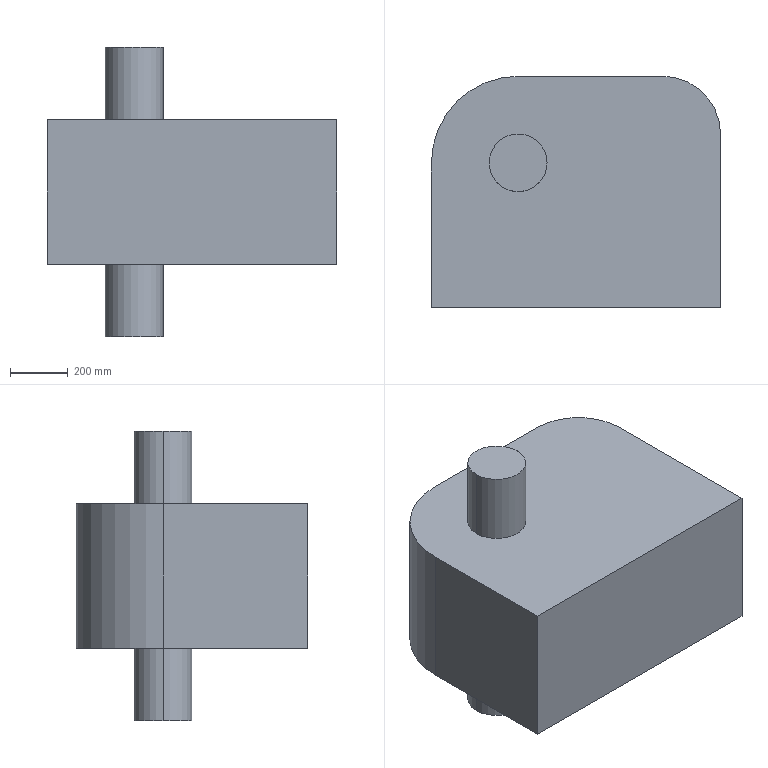Part | SolidWorks | features Fillet 2, Extrusion 1, ICE 1 | 1 solid | 14 faces | box 1000 x 800 x 1000 mm | volume 401758844 mm3 | plane 8 | cylinder 6 | commonest cylinder face diameters 200 x4 400 x1 600 x1
STEP:
#1=CARTESIAN_POINT('',(100.,0.,250.));
#2=VERTEX_POINT('',#1);
#3=CARTESIAN_POINT('',(-100.,0.,250.));
#4=VERTEX_POINT('',#3);
#5=CARTESIAN_POINT('',(0.,0.,250.));
#6=DIRECTION('',(0.,0.,1.));
#7=DIRECTION('',(1.,0.,0.));
#8=AXIS2_PLACEMENT_3D('',#5,#6,#7);
#9=CIRCLE('',#8,100.);
#10=EDGE_CURVE('',#2,#4,#9,.T.);
#11=ORIENTED_EDGE('',*,*,#10,.T.);
#12=CARTESIAN_POINT('',(-100.,0.,500.));
#13=VERTEX_POINT('',#12);
#14=CARTESIAN_POINT('',(-100.,0.,-500.));
#15=DIRECTION('',(0.,0.,1.));
#16=VECTOR('',#15,1000.);
#17=LINE('',#14,#16);
#18=EDGE_CURVE('',#4,#13,#17,.T.);
#19=ORIENTED_EDGE('',*,*,#18,.T.);
#20=CARTESIAN_POINT('',(100.,0.,500.));
#21=VERTEX_POINT('',#20);
#22=CARTESIAN_POINT('',(0.,0.,500.));
#23=DIRECTION('',(0.,0.,1.));
#24=DIRECTION('',(1.,0.,0.));
#25=AXIS2_PLACEMENT_3D('',#22,#23,#24);
#26=CIRCLE('',#25,100.);
#27=EDGE_CURVE('',#21,#13,#26,.T.);
#28=ORIENTED_EDGE('',*,*,#27,.F.);
#29=CARTESIAN_POINT('',(100.,0.,-500.));
#30=DIRECTION('',(0.,0.,1.));
#31=VECTOR('',#30,1000.);
#32=LINE('',#29,#31);
#33=EDGE_CURVE('',#2,#21,#32,.T.);
#34=ORIENTED_EDGE('',*,*,#33,.F.);
#35=EDGE_LOOP('',(#11,#19,#28,#34));
#36=FACE_OUTER_BOUND('',#35,.T.);
#37=CARTESIAN_POINT('',(0.,0.,-500.));
#38=DIRECTION('',(0.,0.,1.));
#39=DIRECTION('',(1.,0.,0.));
#40=AXIS2_PLACEMENT_3D('',#37,#38,#39);
#41=CYLINDRICAL_SURFACE('',#40,100.);
#42=ADVANCED_FACE('',(#36),#41,.T.);
#43=CARTESIAN_POINT('',(100.,0.,-500.));
#44=VERTEX_POINT('',#43);
#45=CARTESIAN_POINT('',(-100.,0.,-500.));
#46=VERTEX_POINT('',#45);
#47=CARTESIAN_POINT('',(0.,0.,-500.));
#48=DIRECTION('',(0.,0.,1.));
#49=DIRECTION('',(1.,0.,0.));
#50=AXIS2_PLACEMENT_3D('',#47,#48,#49);
#51=CIRCLE('',#50,100.);
#52=EDGE_CURVE('',#44,#46,#51,.T.);
#53=ORIENTED_EDGE('',*,*,#52,.T.);
#54=CARTESIAN_POINT('',(-100.,0.,-250.));
#55=VERTEX_POINT('',#54);
#56=CARTESIAN_POINT('',(-100.,0.,-500.));
#57=DIRECTION('',(0.,0.,1.));
#58=VECTOR('',#57,1000.);
#59=LINE('',#56,#58);
#60=EDGE_CURVE('',#46,#55,#59,.T.);
#61=ORIENTED_EDGE('',*,*,#60,.T.);
#62=CARTESIAN_POINT('',(100.,0.,-250.));
#63=VERTEX_POINT('',#62);
#64=CARTESIAN_POINT('',(0.,0.,-250.));
#65=DIRECTION('',(0.,0.,1.));
#66=DIRECTION('',(1.,0.,0.));
#67=AXIS2_PLACEMENT_3D('',#64,#65,#66);
#68=CIRCLE('',#67,100.);
#69=EDGE_CURVE('',#63,#55,#68,.T.);
#70=ORIENTED_EDGE('',*,*,#69,.F.);
#71=CARTESIAN_POINT('',(100.,0.,-500.));
#72=DIRECTION('',(0.,0.,1.));
#73=VECTOR('',#72,1000.);
#74=LINE('',#71,#73);
#75=EDGE_CURVE('',#44,#63,#74,.T.);
#76=ORIENTED_EDGE('',*,*,#75,.F.);
#77=EDGE_LOOP('',(#53,#61,#70,#76));
#78=FACE_OUTER_BOUND('',#77,.T.);
#79=CARTESIAN_POINT('',(0.,0.,-500.));
#80=DIRECTION('',(0.,0.,1.));
#81=DIRECTION('',(1.,0.,0.));
#82=AXIS2_PLACEMENT_3D('',#79,#80,#81);
#83=CYLINDRICAL_SURFACE('',#82,100.);
#84=ADVANCED_FACE('',(#78),#83,.T.);
#85=CARTESIAN_POINT('',(-300.,0.,250.));
#86=VERTEX_POINT('',#85);
#87=CARTESIAN_POINT('',(-300.,-500.,250.));
#88=VERTEX_POINT('',#87);
#89=CARTESIAN_POINT('',(-300.,300.,250.));
#90=DIRECTION('',(0.,-1.,0.));
#91=VECTOR('',#90,1000.);
#92=LINE('',#89,#91);
#93=EDGE_CURVE('',#86,#88,#92,.T.);
#94=ORIENTED_EDGE('',*,*,#93,.F.);
#95=CARTESIAN_POINT('',(-300.,0.,-250.));
#96=VERTEX_POINT('',#95);
#97=CARTESIAN_POINT('',(-300.,0.,250.));
#98=DIRECTION('',(0.,0.,-1.));
#99=VECTOR('',#98,1000.);
#100=LINE('',#97,#99);
#101=EDGE_CURVE('',#86,#96,#100,.T.);
#102=ORIENTED_EDGE('',*,*,#101,.T.);
#103=CARTESIAN_POINT('',(-300.,-500.,-250.));
#104=VERTEX_POINT('',#103);
#105=CARTESIAN_POINT('',(-300.,300.,-250.));
#106=DIRECTION('',(0.,-1.,0.));
#107=VECTOR('',#106,1000.);
#108=LINE('',#105,#107);
#109=EDGE_CURVE('',#96,#104,#108,.T.);
#110=ORIENTED_EDGE('',*,*,#109,.T.);
#111=CARTESIAN_POINT('',(-300.,-500.,250.));
#112=DIRECTION('',(0.,0.,-1.));
#113=VECTOR('',#112,1000.);
#114=LINE('',#111,#113);
#115=EDGE_CURVE('',#88,#104,#114,.T.);
#116=ORIENTED_EDGE('',*,*,#115,.F.);
#117=EDGE_LOOP('',(#94,#102,#110,#116));
#118=FACE_OUTER_BOUND('',#117,.T.);
#119=CARTESIAN_POINT('',(-300.,300.,250.));
#120=DIRECTION('',(1.,0.,0.));
#121=DIRECTION('',(0.,1.,0.));
#122=AXIS2_PLACEMENT_3D('',#119,#120,#121);
#123=PLANE('',#122);
#124=ADVANCED_FACE('',(#118),#123,.F.);
#125=ORIENTED_EDGE('',*,*,#115,.T.);
#126=CARTESIAN_POINT('',(700.,-500.,-250.));
#127=VERTEX_POINT('',#126);
#128=CARTESIAN_POINT('',(-300.,-500.,-250.));
#129=DIRECTION('',(1.,0.,0.));
#130=VECTOR('',#129,1000.);
#131=LINE('',#128,#130);
#132=EDGE_CURVE('',#104,#127,#131,.T.);
#133=ORIENTED_EDGE('',*,*,#132,.T.);
#134=CARTESIAN_POINT('',(700.,-500.,250.));
#135=VERTEX_POINT('',#134);
#136=CARTESIAN_POINT('',(700.,-500.,250.));
#137=DIRECTION('',(0.,0.,-1.));
#138=VECTOR('',#137,1000.);
#139=LINE('',#136,#138);
#140=EDGE_CURVE('',#135,#127,#139,.T.);
#141=ORIENTED_EDGE('',*,*,#140,.F.);
#142=CARTESIAN_POINT('',(-300.,-500.,250.));
#143=DIRECTION('',(1.,0.,0.));
#144=VECTOR('',#143,1000.);
#145=LINE('',#142,#144);
#146=EDGE_CURVE('',#88,#135,#145,.T.);
#147=ORIENTED_EDGE('',*,*,#146,.F.);
#148=EDGE_LOOP('',(#125,#133,#141,#147));
#149=FACE_OUTER_BOUND('',#148,.T.);
#150=CARTESIAN_POINT('',(-300.,-500.,250.));
#151=DIRECTION('',(0.,1.,0.));
#152=DIRECTION('',(0.,0.,1.));
#153=AXIS2_PLACEMENT_3D('',#150,#151,#152);
#154=PLANE('',#153);
#155=ADVANCED_FACE('',(#149),#154,.F.);
#156=CARTESIAN_POINT('',(700.,100.,-250.));
#157=VERTEX_POINT('',#156);
#158=CARTESIAN_POINT('',(700.,300.,-250.));
#159=DIRECTION('',(0.,1.,0.));
#160=VECTOR('',#159,1000.);
#161=LINE('',#158,#160);
#162=EDGE_CURVE('',#127,#157,#161,.T.);
#163=ORIENTED_EDGE('',*,*,#162,.T.);
#164=CARTESIAN_POINT('',(700.,100.,250.));
#165=VERTEX_POINT('',#164);
#166=CARTESIAN_POINT('',(700.,100.,250.));
#167=DIRECTION('',(0.,0.,1.));
#168=VECTOR('',#167,1000.);
#169=LINE('',#166,#168);
#170=EDGE_CURVE('',#157,#165,#169,.T.);
#171=ORIENTED_EDGE('',*,*,#170,.T.);
#172=CARTESIAN_POINT('',(700.,300.,250.));
#173=DIRECTION('',(0.,1.,0.));
#174=VECTOR('',#173,1000.);
#175=LINE('',#172,#174);
#176=EDGE_CURVE('',#135,#165,#175,.T.);
#177=ORIENTED_EDGE('',*,*,#176,.F.);
#178=ORIENTED_EDGE('',*,*,#140,.T.);
#179=EDGE_LOOP('',(#163,#171,#177,#178));
#180=FACE_OUTER_BOUND('',#179,.T.);
#181=CARTESIAN_POINT('',(700.,300.,250.));
#182=DIRECTION('',(-1.,0.,0.));
#183=DIRECTION('',(0.,0.,1.));
#184=AXIS2_PLACEMENT_3D('',#181,#182,#183);
#185=PLANE('',#184);
#186=ADVANCED_FACE('',(#180),#185,.F.);
#187=CARTESIAN_POINT('',(500.,300.,250.));
#188=VERTEX_POINT('',#187);
#189=CARTESIAN_POINT('',(0.,300.,250.));
#190=VERTEX_POINT('',#189);
#191=CARTESIAN_POINT('',(-300.,300.,250.));
#192=DIRECTION('',(-1.,0.,0.));
#193=VECTOR('',#192,1000.);
#194=LINE('',#191,#193);
#195=EDGE_CURVE('',#188,#190,#194,.T.);
#196=ORIENTED_EDGE('',*,*,#195,.F.);
#197=CARTESIAN_POINT('',(500.,300.,-250.));
#198=VERTEX_POINT('',#197);
#199=CARTESIAN_POINT('',(500.,300.,250.));
#200=DIRECTION('',(0.,0.,-1.));
#201=VECTOR('',#200,1000.);
#202=LINE('',#199,#201);
#203=EDGE_CURVE('',#188,#198,#202,.T.);
#204=ORIENTED_EDGE('',*,*,#203,.T.);
#205=CARTESIAN_POINT('',(0.,300.,-250.));
#206=VERTEX_POINT('',#205);
#207=CARTESIAN_POINT('',(-300.,300.,-250.));
#208=DIRECTION('',(-1.,0.,0.));
#209=VECTOR('',#208,1000.);
#210=LINE('',#207,#209);
#211=EDGE_CURVE('',#198,#206,#210,.T.);
#212=ORIENTED_EDGE('',*,*,#211,.T.);
#213=CARTESIAN_POINT('',(0.,300.,250.));
#214=DIRECTION('',(0.,0.,1.));
#215=VECTOR('',#214,1000.);
#216=LINE('',#213,#215);
#217=EDGE_CURVE('',#206,#190,#216,.T.);
#218=ORIENTED_EDGE('',*,*,#217,.T.);
#219=EDGE_LOOP('',(#196,#204,#212,#218));
#220=FACE_OUTER_BOUND('',#219,.T.);
#221=CARTESIAN_POINT('',(-300.,300.,250.));
#222=DIRECTION('',(0.,-1.,0.));
#223=DIRECTION('',(0.,0.,-1.));
#224=AXIS2_PLACEMENT_3D('',#221,#222,#223);
#225=PLANE('',#224);
#226=ADVANCED_FACE('',(#220),#225,.F.);
#227=ORIENTED_EDGE('',*,*,#10,.F.);
#228=CARTESIAN_POINT('',(0.,0.,250.));
#229=DIRECTION('',(0.,0.,1.));
#230=DIRECTION('',(1.,0.,0.));
#231=AXIS2_PLACEMENT_3D('',#228,#229,#230);
#232=CIRCLE('',#231,100.);
#233=EDGE_CURVE('',#4,#2,#232,.T.);
#234=ORIENTED_EDGE('',*,*,#233,.F.);
#235=EDGE_LOOP('',(#227,#234));
#236=FACE_BOUND('',#235,.T.);
#237=ORIENTED_EDGE('',*,*,#176,.T.);
#238=CARTESIAN_POINT('',(500.,100.,250.));
#239=DIRECTION('',(0.,0.,1.));
#240=DIRECTION('',(1.,0.,0.));
#241=AXIS2_PLACEMENT_3D('',#238,#239,#240);
#242=CIRCLE('',#241,200.);
#243=EDGE_CURVE('',#165,#188,#242,.T.);
#244=ORIENTED_EDGE('',*,*,#243,.T.);
#245=ORIENTED_EDGE('',*,*,#195,.T.);
#246=CARTESIAN_POINT('',(0.,0.,250.));
#247=DIRECTION('',(0.,0.,1.));
#248=DIRECTION('',(1.,0.,0.));
#249=AXIS2_PLACEMENT_3D('',#246,#247,#248);
#250=CIRCLE('',#249,300.);
#251=EDGE_CURVE('',#190,#86,#250,.T.);
#252=ORIENTED_EDGE('',*,*,#251,.T.);
#253=ORIENTED_EDGE('',*,*,#93,.T.);
#254=ORIENTED_EDGE('',*,*,#146,.T.);
#255=EDGE_LOOP('',(#237,#244,#245,#252,#253,#254));
#256=FACE_OUTER_BOUND('',#255,.T.);
#257=CARTESIAN_POINT('',(-300.,-500.,250.));
#258=DIRECTION('',(0.,0.,1.));
#259=DIRECTION('',(1.,0.,0.));
#260=AXIS2_PLACEMENT_3D('',#257,#258,#259);
#261=PLANE('',#260);
#262=ADVANCED_FACE('',(#236,#256),#261,.T.);
#263=ORIENTED_EDGE('',*,*,#69,.T.);
#264=CARTESIAN_POINT('',(0.,0.,-250.));
#265=DIRECTION('',(0.,0.,1.));
#266=DIRECTION('',(1.,0.,0.));
#267=AXIS2_PLACEMENT_3D('',#264,#265,#266);
#268=CIRCLE('',#267,100.);
#269=EDGE_CURVE('',#55,#63,#268,.T.);
#270=ORIENTED_EDGE('',*,*,#269,.T.);
#271=EDGE_LOOP('',(#263,#270));
#272=FACE_BOUND('',#271,.T.);
#273=ORIENTED_EDGE('',*,*,#211,.F.);
#274=CARTESIAN_POINT('',(500.,100.,-250.));
#275=DIRECTION('',(0.,0.,-1.));
#276=DIRECTION('',(1.,0.,0.));
#277=AXIS2_PLACEMENT_3D('',#274,#275,#276);
#278=CIRCLE('',#277,200.);
#279=EDGE_CURVE('',#198,#157,#278,.T.);
#280=ORIENTED_EDGE('',*,*,#279,.T.);
#281=ORIENTED_EDGE('',*,*,#162,.F.);
#282=ORIENTED_EDGE('',*,*,#132,.F.);
#283=ORIENTED_EDGE('',*,*,#109,.F.);
#284=CARTESIAN_POINT('',(0.,0.,-250.));
#285=DIRECTION('',(0.,0.,-1.));
#286=DIRECTION('',(1.,0.,0.));
#287=AXIS2_PLACEMENT_3D('',#284,#285,#286);
#288=CIRCLE('',#287,300.);
#289=EDGE_CURVE('',#96,#206,#288,.T.);
#290=ORIENTED_EDGE('',*,*,#289,.T.);
#291=EDGE_LOOP('',(#273,#280,#281,#282,#283,#290));
#292=FACE_OUTER_BOUND('',#291,.T.);
#293=CARTESIAN_POINT('',(-300.,-500.,-250.));
#294=DIRECTION('',(0.,0.,1.));
#295=DIRECTION('',(1.,0.,0.));
#296=AXIS2_PLACEMENT_3D('',#293,#294,#295);
#297=PLANE('',#296);
#298=ADVANCED_FACE('',(#272,#292),#297,.F.);
#299=ORIENTED_EDGE('',*,*,#52,.F.);
#300=CARTESIAN_POINT('',(0.,0.,-500.));
#301=DIRECTION('',(0.,0.,1.));
#302=DIRECTION('',(1.,0.,0.));
#303=AXIS2_PLACEMENT_3D('',#300,#301,#302);
#304=CIRCLE('',#303,100.);
#305=EDGE_CURVE('',#46,#44,#304,.T.);
#306=ORIENTED_EDGE('',*,*,#305,.F.);
#307=EDGE_LOOP('',(#299,#306));
#308=FACE_OUTER_BOUND('',#307,.T.);
#309=CARTESIAN_POINT('',(0.,0.,-500.));
#310=DIRECTION('',(0.,0.,1.));
#311=DIRECTION('',(1.,0.,0.));
#312=AXIS2_PLACEMENT_3D('',#309,#310,#311);
#313=PLANE('',#312);
#314=ADVANCED_FACE('',(#308),#313,.F.);
#315=ORIENTED_EDGE('',*,*,#60,.F.);
#316=ORIENTED_EDGE('',*,*,#305,.T.);
#317=ORIENTED_EDGE('',*,*,#75,.T.);
#318=ORIENTED_EDGE('',*,*,#269,.F.);
#319=EDGE_LOOP('',(#315,#316,#317,#318));
#320=FACE_OUTER_BOUND('',#319,.T.);
#321=CARTESIAN_POINT('',(0.,0.,-500.));
#322=DIRECTION('',(0.,0.,1.));
#323=DIRECTION('',(1.,0.,0.));
#324=AXIS2_PLACEMENT_3D('',#321,#322,#323);
#325=CYLINDRICAL_SURFACE('',#324,100.);
#326=ADVANCED_FACE('',(#320),#325,.T.);
#327=ORIENTED_EDGE('',*,*,#18,.F.);
#328=ORIENTED_EDGE('',*,*,#233,.T.);
#329=ORIENTED_EDGE('',*,*,#33,.T.);
#330=CARTESIAN_POINT('',(0.,0.,500.));
#331=DIRECTION('',(0.,0.,1.));
#332=DIRECTION('',(1.,0.,0.));
#333=AXIS2_PLACEMENT_3D('',#330,#331,#332);
#334=CIRCLE('',#333,100.);
#335=EDGE_CURVE('',#13,#21,#334,.T.);
#336=ORIENTED_EDGE('',*,*,#335,.F.);
#337=EDGE_LOOP('',(#327,#328,#329,#336));
#338=FACE_OUTER_BOUND('',#337,.T.);
#339=CARTESIAN_POINT('',(0.,0.,-500.));
#340=DIRECTION('',(0.,0.,1.));
#341=DIRECTION('',(1.,0.,0.));
#342=AXIS2_PLACEMENT_3D('',#339,#340,#341);
#343=CYLINDRICAL_SURFACE('',#342,100.);
#344=ADVANCED_FACE('',(#338),#343,.T.);
#345=ORIENTED_EDGE('',*,*,#27,.T.);
#346=ORIENTED_EDGE('',*,*,#335,.T.);
#347=EDGE_LOOP('',(#345,#346));
#348=FACE_OUTER_BOUND('',#347,.T.);
#349=CARTESIAN_POINT('',(0.,0.,500.));
#350=DIRECTION('',(0.,0.,1.));
#351=DIRECTION('',(1.,0.,0.));
#352=AXIS2_PLACEMENT_3D('',#349,#350,#351);
#353=PLANE('',#352);
#354=ADVANCED_FACE('',(#348),#353,.T.);
#355=ORIENTED_EDGE('',*,*,#251,.F.);
#356=ORIENTED_EDGE('',*,*,#217,.F.);
#357=ORIENTED_EDGE('',*,*,#289,.F.);
#358=ORIENTED_EDGE('',*,*,#101,.F.);
#359=EDGE_LOOP('',(#355,#356,#357,#358));
#360=FACE_OUTER_BOUND('',#359,.T.);
#361=CARTESIAN_POINT('',(0.,0.,250.));
#362=DIRECTION('',(0.,0.,-1.));
#363=DIRECTION('',(-1.,0.,0.));
#364=AXIS2_PLACEMENT_3D('',#361,#362,#363);
#365=CYLINDRICAL_SURFACE('',#364,300.);
#366=ADVANCED_FACE('',(#360),#365,.T.);
#367=ORIENTED_EDGE('',*,*,#243,.F.);
#368=ORIENTED_EDGE('',*,*,#170,.F.);
#369=ORIENTED_EDGE('',*,*,#279,.F.);
#370=ORIENTED_EDGE('',*,*,#203,.F.);
#371=EDGE_LOOP('',(#367,#368,#369,#370));
#372=FACE_OUTER_BOUND('',#371,.T.);
#373=CARTESIAN_POINT('',(500.,100.,250.));
#374=DIRECTION('',(0.,0.,-1.));
#375=DIRECTION('',(-1.,0.,0.));
#376=AXIS2_PLACEMENT_3D('',#373,#374,#375);
#377=CYLINDRICAL_SURFACE('',#376,200.);
#378=ADVANCED_FACE('',(#372),#377,.T.);
#379=CLOSED_SHELL('',(#42,#84,#124,#155,#186,#226,#262,#298,#314,#326,#344,#354,#366,#378));
#380=MANIFOLD_SOLID_BREP('',#379);
#381=CARTESIAN_POINT('',(0.,0.,0.));
#382=DIRECTION('',(0.,0.,1.));
#383=DIRECTION('',(1.,0.,0.));
#384=AXIS2_PLACEMENT_3D('',#381,#382,#383);
#385=(LENGTH_UNIT()NAMED_UNIT(*)SI_UNIT(.MILLI.,.METRE.));
#386=UNCERTAINTY_MEASURE_WITH_UNIT(LENGTH_MEASURE(0.00001),#385,'','');
#387=(NAMED_UNIT(*)PLANE_ANGLE_UNIT()SI_UNIT($,.RADIAN.));
#388=(NAMED_UNIT(*)SI_UNIT($,.STERADIAN.)SOLID_ANGLE_UNIT());
#389=(GEOMETRIC_REPRESENTATION_CONTEXT(3)GLOBAL_UNCERTAINTY_ASSIGNED_CONTEXT((#386))GLOBAL_UNIT_ASSIGNED_CONTEXT((#385,#387,#388))REPRESENTATION_CONTEXT('',''));
#390=ADVANCED_BREP_SHAPE_REPRESENTATION('',(#380,#384),#389);